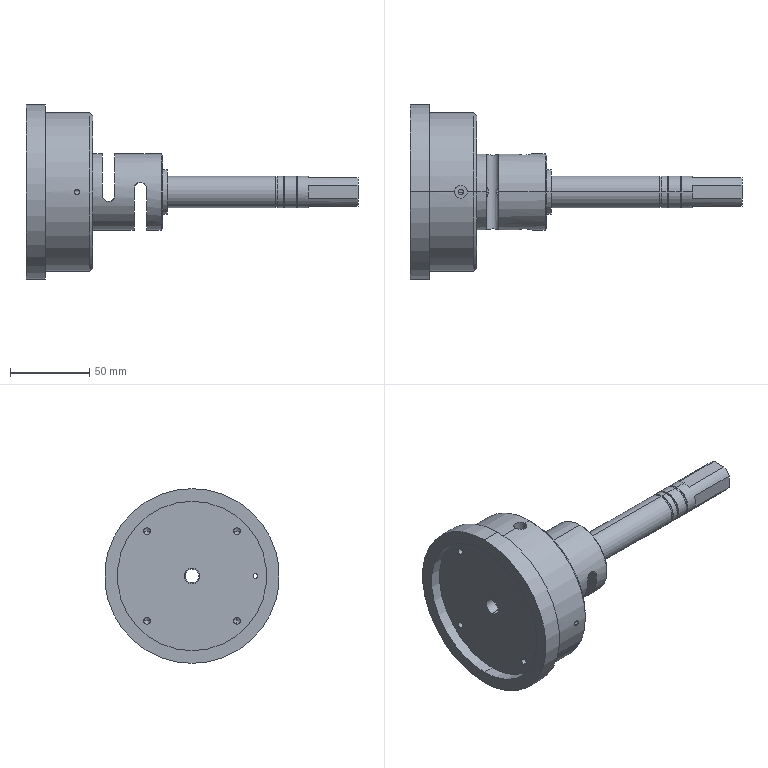Part | STEP file | longitudinal seal wheel_SUS304 | 2 solids | 100 faces | box 209 x 110 x 110 mm | volume 385908 mm3 | cylinder 58 | plane 30 | cone 12 | commonest cylinder face diameters 3.3 x8 4.2 x8 20 x8 10 x6 18.85 x6 8 x5